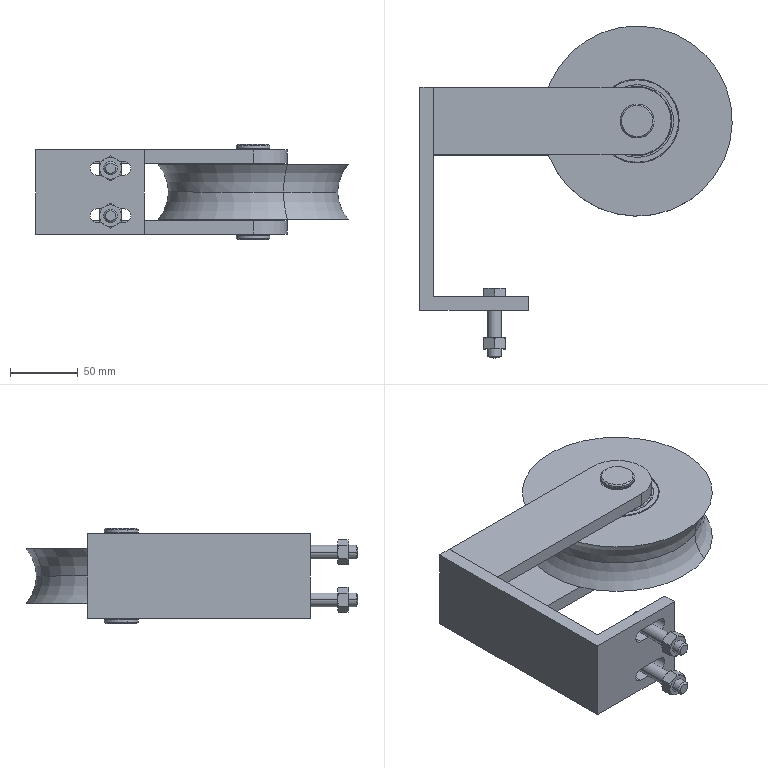Part | SolidWorks | features ReferencePattern 2, LocalLPattern 1 | 11 solids | 344 faces | box 230 x 244.4 x 70 mm | volume 814861 mm3 | torus 108 | plane 76 | cylinder 64 | sphere 52 | cone 44 | commonest cylinder face diameters 25 x14 10 x12 37.333 x8 62 x6 14.4 x4 23.9 x4